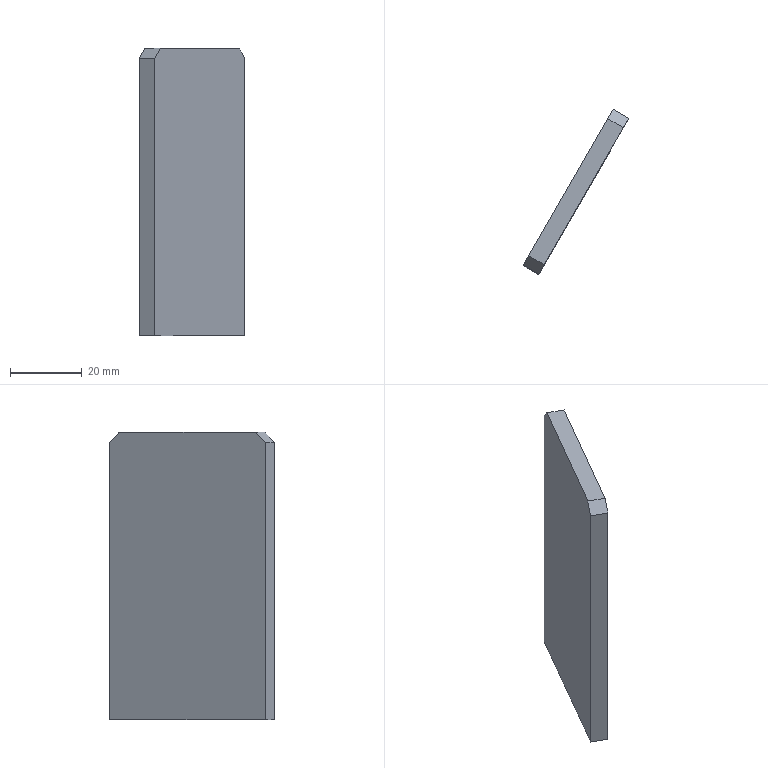Part | SolidWorks | features BaseBody 1 | 1 solid | 8 faces | box 29.33 x 45.801 x 80 mm | volume 19955 mm3 | plane 8
STEP:
#1=CARTESIAN_POINT('',(-206.909,1743.519,-330.));
#2=VERTEX_POINT('',#1);
#3=CARTESIAN_POINT('',(-205.409,1746.117,-327.));
#4=VERTEX_POINT('',#3);
#5=CARTESIAN_POINT('',(-206.909,1743.519,-330.));
#6=DIRECTION('',(0.3536,0.6124,0.7071));
#7=VECTOR('',#6,1000.);
#8=LINE('',#5,#7);
#9=EDGE_CURVE('',#2,#4,#8,.T.);
#10=ORIENTED_EDGE('',*,*,#9,.T.);
#11=CARTESIAN_POINT('',(-183.409,1784.222,-327.));
#12=VERTEX_POINT('',#11);
#13=CARTESIAN_POINT('',(-194.409,1765.17,-327.));
#14=DIRECTION('',(0.5,0.866,0.));
#15=VECTOR('',#14,1000.);
#16=LINE('',#13,#15);
#17=EDGE_CURVE('',#4,#12,#16,.T.);
#18=ORIENTED_EDGE('',*,*,#17,.T.);
#19=CARTESIAN_POINT('',(-181.909,1786.82,-330.));
#20=VERTEX_POINT('',#19);
#21=CARTESIAN_POINT('',(-183.409,1784.222,-327.));
#22=DIRECTION('',(0.3536,0.6124,-0.7071));
#23=VECTOR('',#22,1000.);
#24=LINE('',#21,#23);
#25=EDGE_CURVE('',#12,#20,#24,.T.);
#26=ORIENTED_EDGE('',*,*,#25,.T.);
#27=CARTESIAN_POINT('',(-181.909,1786.82,-407.));
#28=VERTEX_POINT('',#27);
#29=CARTESIAN_POINT('',(-181.909,1786.82,-367.));
#30=DIRECTION('',(0.,0.,-1.));
#31=VECTOR('',#30,1000.);
#32=LINE('',#29,#31);
#33=EDGE_CURVE('',#20,#28,#32,.T.);
#34=ORIENTED_EDGE('',*,*,#33,.T.);
#35=CARTESIAN_POINT('',(-206.909,1743.519,-407.));
#36=VERTEX_POINT('',#35);
#37=CARTESIAN_POINT('',(-194.409,1765.17,-407.));
#38=DIRECTION('',(-0.5,-0.866,0.));
#39=VECTOR('',#38,1000.);
#40=LINE('',#37,#39);
#41=EDGE_CURVE('',#28,#36,#40,.T.);
#42=ORIENTED_EDGE('',*,*,#41,.T.);
#43=CARTESIAN_POINT('',(-206.909,1743.519,-367.));
#44=DIRECTION('',(0.,0.,1.));
#45=VECTOR('',#44,1000.);
#46=LINE('',#43,#45);
#47=EDGE_CURVE('',#36,#2,#46,.T.);
#48=ORIENTED_EDGE('',*,*,#47,.T.);
#49=EDGE_LOOP('',(#10,#18,#26,#34,#42,#48));
#50=FACE_OUTER_BOUND('',#49,.T.);
#51=CARTESIAN_POINT('',(-194.409,1765.17,-367.));
#52=DIRECTION('',(-0.866,0.5,0.));
#53=DIRECTION('',(-0.5,-0.866,0.));
#54=AXIS2_PLACEMENT_3D('',#51,#52,#53);
#55=PLANE('',#54);
#56=ADVANCED_FACE('',(#50),#55,.T.);
#57=CARTESIAN_POINT('',(-201.079,1743.617,-327.));
#58=VERTEX_POINT('',#57);
#59=CARTESIAN_POINT('',(-205.409,1746.117,-327.));
#60=DIRECTION('',(0.866,-0.5,0.));
#61=VECTOR('',#60,1000.);
#62=LINE('',#59,#61);
#63=EDGE_CURVE('',#4,#58,#62,.T.);
#64=ORIENTED_EDGE('',*,*,#63,.T.);
#65=CARTESIAN_POINT('',(-179.079,1781.722,-327.));
#66=VERTEX_POINT('',#65);
#67=CARTESIAN_POINT('',(-201.079,1743.617,-327.));
#68=DIRECTION('',(0.5,0.866,0.));
#69=VECTOR('',#68,1000.);
#70=LINE('',#67,#69);
#71=EDGE_CURVE('',#58,#66,#70,.T.);
#72=ORIENTED_EDGE('',*,*,#71,.T.);
#73=CARTESIAN_POINT('',(-179.079,1781.722,-327.));
#74=DIRECTION('',(-0.866,0.5,0.));
#75=VECTOR('',#74,1000.);
#76=LINE('',#73,#75);
#77=EDGE_CURVE('',#66,#12,#76,.T.);
#78=ORIENTED_EDGE('',*,*,#77,.T.);
#79=ORIENTED_EDGE('',*,*,#17,.F.);
#80=EDGE_LOOP('',(#64,#72,#78,#79));
#81=FACE_OUTER_BOUND('',#80,.T.);
#82=CARTESIAN_POINT('',(-202.579,1741.019,-327.));
#83=DIRECTION('',(0.,0.,1.));
#84=DIRECTION('',(1.,0.,0.));
#85=AXIS2_PLACEMENT_3D('',#82,#83,#84);
#86=PLANE('',#85);
#87=ADVANCED_FACE('',(#81),#86,.T.);
#88=ORIENTED_EDGE('',*,*,#9,.F.);
#89=CARTESIAN_POINT('',(-202.579,1741.019,-330.));
#90=VERTEX_POINT('',#89);
#91=CARTESIAN_POINT('',(-202.579,1741.019,-330.));
#92=DIRECTION('',(-0.866,0.5,0.));
#93=VECTOR('',#92,1000.);
#94=LINE('',#91,#93);
#95=EDGE_CURVE('',#90,#2,#94,.T.);
#96=ORIENTED_EDGE('',*,*,#95,.F.);
#97=CARTESIAN_POINT('',(-201.079,1743.617,-327.));
#98=DIRECTION('',(-0.3536,-0.6124,-0.7071));
#99=VECTOR('',#98,1000.);
#100=LINE('',#97,#99);
#101=EDGE_CURVE('',#58,#90,#100,.T.);
#102=ORIENTED_EDGE('',*,*,#101,.F.);
#103=ORIENTED_EDGE('',*,*,#63,.F.);
#104=EDGE_LOOP('',(#88,#96,#102,#103));
#105=FACE_OUTER_BOUND('',#104,.T.);
#106=CARTESIAN_POINT('',(-202.579,1741.019,-330.));
#107=DIRECTION('',(0.3536,0.6124,-0.7071));
#108=DIRECTION('',(0.,0.7559,0.6547));
#109=AXIS2_PLACEMENT_3D('',#106,#107,#108);
#110=PLANE('',#109);
#111=ADVANCED_FACE('',(#105),#110,.F.);
#112=CARTESIAN_POINT('',(-202.579,1741.019,-407.));
#113=VERTEX_POINT('',#112);
#114=CARTESIAN_POINT('',(-202.579,1741.019,-407.));
#115=DIRECTION('',(0.866,-0.5,0.));
#116=VECTOR('',#115,1000.);
#117=LINE('',#114,#116);
#118=EDGE_CURVE('',#36,#113,#117,.T.);
#119=ORIENTED_EDGE('',*,*,#118,.T.);
#120=CARTESIAN_POINT('',(-202.579,1741.019,-407.));
#121=DIRECTION('',(0.,0.,1.));
#122=VECTOR('',#121,1000.);
#123=LINE('',#120,#122);
#124=EDGE_CURVE('',#113,#90,#123,.T.);
#125=ORIENTED_EDGE('',*,*,#124,.T.);
#126=ORIENTED_EDGE('',*,*,#95,.T.);
#127=ORIENTED_EDGE('',*,*,#47,.F.);
#128=EDGE_LOOP('',(#119,#125,#126,#127));
#129=FACE_OUTER_BOUND('',#128,.T.);
#130=CARTESIAN_POINT('',(-202.579,1741.019,-407.));
#131=DIRECTION('',(-0.5,-0.866,0.));
#132=DIRECTION('',(0.866,-0.5,0.));
#133=AXIS2_PLACEMENT_3D('',#130,#131,#132);
#134=PLANE('',#133);
#135=ADVANCED_FACE('',(#129),#134,.T.);
#136=ORIENTED_EDGE('',*,*,#118,.F.);
#137=ORIENTED_EDGE('',*,*,#41,.F.);
#138=CARTESIAN_POINT('',(-177.579,1784.32,-407.));
#139=VERTEX_POINT('',#138);
#140=CARTESIAN_POINT('',(-181.909,1786.82,-407.));
#141=DIRECTION('',(0.866,-0.5,0.));
#142=VECTOR('',#141,1000.);
#143=LINE('',#140,#142);
#144=EDGE_CURVE('',#28,#139,#143,.T.);
#145=ORIENTED_EDGE('',*,*,#144,.T.);
#146=CARTESIAN_POINT('',(-177.579,1784.32,-407.));
#147=DIRECTION('',(-0.5,-0.866,0.));
#148=VECTOR('',#147,1000.);
#149=LINE('',#146,#148);
#150=EDGE_CURVE('',#139,#113,#149,.T.);
#151=ORIENTED_EDGE('',*,*,#150,.T.);
#152=EDGE_LOOP('',(#136,#137,#145,#151));
#153=FACE_OUTER_BOUND('',#152,.T.);
#154=CARTESIAN_POINT('',(-202.579,1741.019,-407.));
#155=DIRECTION('',(0.,0.,-1.));
#156=DIRECTION('',(-1.,0.,0.));
#157=AXIS2_PLACEMENT_3D('',#154,#155,#156);
#158=PLANE('',#157);
#159=ADVANCED_FACE('',(#153),#158,.T.);
#160=ORIENTED_EDGE('',*,*,#144,.F.);
#161=ORIENTED_EDGE('',*,*,#33,.F.);
#162=CARTESIAN_POINT('',(-177.579,1784.32,-330.));
#163=VERTEX_POINT('',#162);
#164=CARTESIAN_POINT('',(-177.579,1784.32,-330.));
#165=DIRECTION('',(0.866,-0.5,0.));
#166=VECTOR('',#165,1000.);
#167=LINE('',#164,#166);
#168=EDGE_CURVE('',#20,#163,#167,.T.);
#169=ORIENTED_EDGE('',*,*,#168,.T.);
#170=CARTESIAN_POINT('',(-177.579,1784.32,-407.));
#171=DIRECTION('',(0.,0.,-1.));
#172=VECTOR('',#171,1000.);
#173=LINE('',#170,#172);
#174=EDGE_CURVE('',#163,#139,#173,.T.);
#175=ORIENTED_EDGE('',*,*,#174,.T.);
#176=EDGE_LOOP('',(#160,#161,#169,#175));
#177=FACE_OUTER_BOUND('',#176,.T.);
#178=CARTESIAN_POINT('',(-177.579,1784.32,-407.));
#179=DIRECTION('',(0.5,0.866,0.));
#180=DIRECTION('',(-0.866,0.5,0.));
#181=AXIS2_PLACEMENT_3D('',#178,#179,#180);
#182=PLANE('',#181);
#183=ADVANCED_FACE('',(#177),#182,.T.);
#184=ORIENTED_EDGE('',*,*,#25,.F.);
#185=ORIENTED_EDGE('',*,*,#77,.F.);
#186=CARTESIAN_POINT('',(-177.579,1784.32,-330.));
#187=DIRECTION('',(-0.3536,-0.6124,0.7071));
#188=VECTOR('',#187,1000.);
#189=LINE('',#186,#188);
#190=EDGE_CURVE('',#163,#66,#189,.T.);
#191=ORIENTED_EDGE('',*,*,#190,.F.);
#192=ORIENTED_EDGE('',*,*,#168,.F.);
#193=EDGE_LOOP('',(#184,#185,#191,#192));
#194=FACE_OUTER_BOUND('',#193,.T.);
#195=CARTESIAN_POINT('',(-179.079,1781.722,-327.));
#196=DIRECTION('',(-0.3536,-0.6124,-0.7071));
#197=DIRECTION('',(0.,0.7559,-0.6547));
#198=AXIS2_PLACEMENT_3D('',#195,#196,#197);
#199=PLANE('',#198);
#200=ADVANCED_FACE('',(#194),#199,.F.);
#201=ORIENTED_EDGE('',*,*,#71,.F.);
#202=ORIENTED_EDGE('',*,*,#101,.T.);
#203=ORIENTED_EDGE('',*,*,#124,.F.);
#204=ORIENTED_EDGE('',*,*,#150,.F.);
#205=ORIENTED_EDGE('',*,*,#174,.F.);
#206=ORIENTED_EDGE('',*,*,#190,.T.);
#207=EDGE_LOOP('',(#201,#202,#203,#204,#205,#206));
#208=FACE_OUTER_BOUND('',#207,.T.);
#209=CARTESIAN_POINT('',(-190.079,1762.67,-367.));
#210=DIRECTION('',(-0.866,0.5,0.));
#211=DIRECTION('',(-0.5,-0.866,0.));
#212=AXIS2_PLACEMENT_3D('',#209,#210,#211);
#213=PLANE('',#212);
#214=ADVANCED_FACE('',(#208),#213,.F.);
#215=CLOSED_SHELL('',(#56,#87,#111,#135,#159,#183,#200,#214));
#216=MANIFOLD_SOLID_BREP('',#215);
#217=CARTESIAN_POINT('',(0.,0.,0.));
#218=DIRECTION('',(0.,0.,1.));
#219=DIRECTION('',(1.,0.,0.));
#220=AXIS2_PLACEMENT_3D('',#217,#218,#219);
#221=(LENGTH_UNIT()NAMED_UNIT(*)SI_UNIT(.MILLI.,.METRE.));
#222=UNCERTAINTY_MEASURE_WITH_UNIT(LENGTH_MEASURE(0.00001),#221,'','');
#223=(NAMED_UNIT(*)PLANE_ANGLE_UNIT()SI_UNIT($,.RADIAN.));
#224=(NAMED_UNIT(*)SI_UNIT($,.STERADIAN.)SOLID_ANGLE_UNIT());
#225=(GEOMETRIC_REPRESENTATION_CONTEXT(3)GLOBAL_UNCERTAINTY_ASSIGNED_CONTEXT((#222))GLOBAL_UNIT_ASSIGNED_CONTEXT((#221,#223,#224))REPRESENTATION_CONTEXT('',''));
#226=ADVANCED_BREP_SHAPE_REPRESENTATION('',(#216,#220),#225);